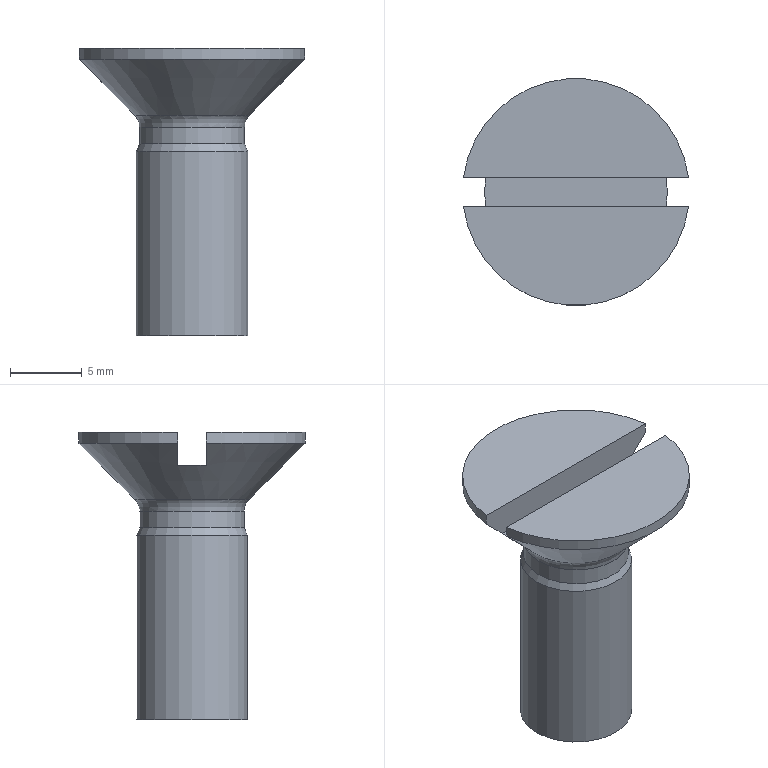Part | NX | features DATUM_CSYS 2, SKETCH 2, EXTRUDE 1, LINE 1, META 1, SWP104 1, SYMBOLIC_THREAD 1, THREADS 1 | 1 solid | 13 faces | box 15.673 x 15.8 x 20 mm | volume 1245 mm3 | plane 6 | cylinder 4 | cone 2 | torus 1 | commonest cylinder face diameters 15.8 x2 7.309 x1 7.76 x1
STEP:
#1=CARTESIAN_POINT('',(7.836,1.,0.));
#2=VERTEX_POINT('',#1);
#3=CARTESIAN_POINT('',(-7.836,1.,0.));
#4=VERTEX_POINT('',#3);
#5=CARTESIAN_POINT('',(17.3,1.,0.));
#6=DIRECTION('',(-1.,0.,0.));
#7=VECTOR('',#6,1000.);
#8=LINE('',#5,#7);
#9=EDGE_CURVE('',#2,#4,#8,.T.);
#10=ORIENTED_EDGE('',*,*,#9,.F.);
#11=CARTESIAN_POINT('',(0.,0.,0.));
#12=DIRECTION('',(0.,0.,-1.));
#13=DIRECTION('',(-1.,0.,0.));
#14=AXIS2_PLACEMENT_3D('',#11,#12,#13);
#15=CIRCLE('',#14,7.9);
#16=EDGE_CURVE('',#4,#2,#15,.T.);
#17=ORIENTED_EDGE('',*,*,#16,.F.);
#18=EDGE_LOOP('',(#10,#17));
#19=FACE_BOUND('',#18,.T.);
#20=CARTESIAN_POINT('',(0.,0.,0.));
#21=DIRECTION('',(0.,0.,-1.));
#22=DIRECTION('',(-1.,0.,0.));
#23=AXIS2_PLACEMENT_3D('',#20,#21,#22);
#24=PLANE('',#23);
#25=ADVANCED_FACE('',(#19),#24,.F.);
#26=ORIENTED_EDGE('',*,*,#16,.T.);
#27=CARTESIAN_POINT('',(7.836,1.,-0.75));
#28=VERTEX_POINT('',#27);
#29=CARTESIAN_POINT('',(7.836,1.,0.));
#30=DIRECTION('',(0.,0.,-1.));
#31=VECTOR('',#30,1000.);
#32=LINE('',#29,#31);
#33=EDGE_CURVE('',#2,#28,#32,.T.);
#34=ORIENTED_EDGE('',*,*,#33,.T.);
#35=CARTESIAN_POINT('',(-7.836,1.,-0.75));
#36=VERTEX_POINT('',#35);
#37=CARTESIAN_POINT('',(0.,0.,-0.75));
#38=DIRECTION('',(0.,0.,-1.));
#39=DIRECTION('',(-1.,0.,0.));
#40=AXIS2_PLACEMENT_3D('',#37,#38,#39);
#41=CIRCLE('',#40,7.9);
#42=EDGE_CURVE('',#36,#28,#41,.T.);
#43=ORIENTED_EDGE('',*,*,#42,.F.);
#44=CARTESIAN_POINT('',(-7.836,1.,0.));
#45=DIRECTION('',(0.,0.,-1.));
#46=VECTOR('',#45,1000.);
#47=LINE('',#44,#46);
#48=EDGE_CURVE('',#36,#4,#47,.F.);
#49=ORIENTED_EDGE('',*,*,#48,.T.);
#50=EDGE_LOOP('',(#26,#34,#43,#49));
#51=FACE_BOUND('',#50,.T.);
#52=CARTESIAN_POINT('',(0.,0.,0.));
#53=DIRECTION('',(0.,0.,-1.));
#54=DIRECTION('',(-1.,0.,0.));
#55=AXIS2_PLACEMENT_3D('',#52,#53,#54);
#56=CYLINDRICAL_SURFACE('',#55,7.9);
#57=ADVANCED_FACE('',(#51),#56,.T.);
#58=CARTESIAN_POINT('',(-3.88,0.,-7.15));
#59=VERTEX_POINT('',#58);
#60=CARTESIAN_POINT('',(0.,0.,-7.15));
#61=DIRECTION('',(0.,0.,-1.));
#62=DIRECTION('',(-1.,0.,0.));
#63=AXIS2_PLACEMENT_3D('',#60,#61,#62);
#64=CIRCLE('',#63,3.88);
#65=EDGE_CURVE('',#59,#59,#64,.T.);
#66=ORIENTED_EDGE('',*,*,#65,.F.);
#67=EDGE_LOOP('',(#66));
#68=FACE_BOUND('',#67,.T.);
#69=CARTESIAN_POINT('',(-3.655,0.,-6.65));
#70=VERTEX_POINT('',#69);
#71=CARTESIAN_POINT('',(0.,0.,-6.65));
#72=DIRECTION('',(0.,0.,-1.));
#73=DIRECTION('',(-1.,0.,0.));
#74=AXIS2_PLACEMENT_3D('',#71,#72,#73);
#75=CIRCLE('',#74,3.655);
#76=EDGE_CURVE('',#70,#70,#75,.T.);
#77=ORIENTED_EDGE('',*,*,#76,.T.);
#78=EDGE_LOOP('',(#77));
#79=FACE_BOUND('',#78,.T.);
#80=CARTESIAN_POINT('',(0.,0.,-6.65));
#81=DIRECTION('',(0.,0.,-1.));
#82=DIRECTION('',(-1.,0.,0.));
#83=AXIS2_PLACEMENT_3D('',#80,#81,#82);
#84=CONICAL_SURFACE('',#83,3.655,0.4233);
#85=ADVANCED_FACE('',(#68,#79),#84,.T.);
#86=CARTESIAN_POINT('',(-3.88,0.,-20.));
#87=VERTEX_POINT('',#86);
#88=CARTESIAN_POINT('',(0.,0.,-20.));
#89=DIRECTION('',(0.,0.,-1.));
#90=DIRECTION('',(-1.,0.,0.));
#91=AXIS2_PLACEMENT_3D('',#88,#89,#90);
#92=CIRCLE('',#91,3.88);
#93=EDGE_CURVE('',#87,#87,#92,.T.);
#94=ORIENTED_EDGE('',*,*,#93,.F.);
#95=EDGE_LOOP('',(#94));
#96=FACE_BOUND('',#95,.T.);
#97=ORIENTED_EDGE('',*,*,#65,.T.);
#98=EDGE_LOOP('',(#97));
#99=FACE_BOUND('',#98,.T.);
#100=CARTESIAN_POINT('',(0.,0.,0.));
#101=DIRECTION('',(0.,0.,-1.));
#102=DIRECTION('',(-1.,0.,0.));
#103=AXIS2_PLACEMENT_3D('',#100,#101,#102);
#104=CYLINDRICAL_SURFACE('',#103,3.88);
#105=ADVANCED_FACE('',(#96,#99),#104,.T.);
#106=ORIENTED_EDGE('',*,*,#93,.T.);
#107=EDGE_LOOP('',(#106));
#108=FACE_BOUND('',#107,.T.);
#109=CARTESIAN_POINT('',(0.,3.88,-20.));
#110=DIRECTION('',(0.,0.,1.));
#111=DIRECTION('',(1.,0.,0.));
#112=AXIS2_PLACEMENT_3D('',#109,#110,#111);
#113=PLANE('',#112);
#114=ADVANCED_FACE('',(#108),#113,.F.);
#115=CARTESIAN_POINT('',(7.836,-1.,0.));
#116=VERTEX_POINT('',#115);
#117=CARTESIAN_POINT('',(-7.836,-1.,0.));
#118=VERTEX_POINT('',#117);
#119=CARTESIAN_POINT('',(0.,0.,0.));
#120=DIRECTION('',(0.,0.,-1.));
#121=DIRECTION('',(-1.,0.,0.));
#122=AXIS2_PLACEMENT_3D('',#119,#120,#121);
#123=CIRCLE('',#122,7.9);
#124=EDGE_CURVE('',#116,#118,#123,.T.);
#125=ORIENTED_EDGE('',*,*,#124,.F.);
#126=CARTESIAN_POINT('',(17.3,-1.,0.));
#127=DIRECTION('',(-1.,0.,0.));
#128=VECTOR('',#127,1000.);
#129=LINE('',#126,#128);
#130=EDGE_CURVE('',#116,#118,#129,.T.);
#131=ORIENTED_EDGE('',*,*,#130,.T.);
#132=EDGE_LOOP('',(#125,#131));
#133=FACE_BOUND('',#132,.T.);
#134=CARTESIAN_POINT('',(0.,0.,0.));
#135=DIRECTION('',(0.,0.,-1.));
#136=DIRECTION('',(-1.,0.,0.));
#137=AXIS2_PLACEMENT_3D('',#134,#135,#136);
#138=PLANE('',#137);
#139=ADVANCED_FACE('',(#133),#138,.F.);
#140=ORIENTED_EDGE('',*,*,#124,.T.);
#141=CARTESIAN_POINT('',(-7.836,-1.,-0.75));
#142=VERTEX_POINT('',#141);
#143=CARTESIAN_POINT('',(-7.836,-1.,0.));
#144=DIRECTION('',(0.,0.,-1.));
#145=VECTOR('',#144,1000.);
#146=LINE('',#143,#145);
#147=EDGE_CURVE('',#118,#142,#146,.T.);
#148=ORIENTED_EDGE('',*,*,#147,.T.);
#149=CARTESIAN_POINT('',(7.836,-1.,-0.75));
#150=VERTEX_POINT('',#149);
#151=CARTESIAN_POINT('',(0.,0.,-0.75));
#152=DIRECTION('',(0.,0.,-1.));
#153=DIRECTION('',(-1.,0.,0.));
#154=AXIS2_PLACEMENT_3D('',#151,#152,#153);
#155=CIRCLE('',#154,7.9);
#156=EDGE_CURVE('',#150,#142,#155,.T.);
#157=ORIENTED_EDGE('',*,*,#156,.F.);
#158=CARTESIAN_POINT('',(7.836,-1.,0.));
#159=DIRECTION('',(0.,0.,-1.));
#160=VECTOR('',#159,1000.);
#161=LINE('',#158,#160);
#162=EDGE_CURVE('',#150,#116,#161,.F.);
#163=ORIENTED_EDGE('',*,*,#162,.T.);
#164=EDGE_LOOP('',(#140,#148,#157,#163));
#165=FACE_BOUND('',#164,.T.);
#166=CARTESIAN_POINT('',(0.,0.,0.));
#167=DIRECTION('',(0.,0.,-1.));
#168=DIRECTION('',(-1.,0.,0.));
#169=AXIS2_PLACEMENT_3D('',#166,#167,#168);
#170=CYLINDRICAL_SURFACE('',#169,7.9);
#171=ADVANCED_FACE('',(#165),#170,.T.);
#172=CARTESIAN_POINT('',(-4.,0.,-4.65));
#173=VERTEX_POINT('',#172);
#174=CARTESIAN_POINT('',(0.,0.,-4.65));
#175=DIRECTION('',(0.,0.,-1.));
#176=DIRECTION('',(-1.,0.,0.));
#177=AXIS2_PLACEMENT_3D('',#174,#175,#176);
#178=CIRCLE('',#177,4.);
#179=EDGE_CURVE('',#173,#173,#178,.T.);
#180=ORIENTED_EDGE('',*,*,#179,.F.);
#181=EDGE_LOOP('',(#180));
#182=FACE_BOUND('',#181,.T.);
#183=CARTESIAN_POINT('',(-6.271,-1.,-2.3));
#184=VERTEX_POINT('',#183);
#185=CARTESIAN_POINT('',(-6.271,1.,-2.3));
#186=VERTEX_POINT('',#185);
#187=CARTESIAN_POINT('',(0.,0.,-2.3));
#188=DIRECTION('',(0.,0.,-1.));
#189=DIRECTION('',(0.,1.,0.));
#190=AXIS2_PLACEMENT_3D('',#187,#188,#189);
#191=CIRCLE('',#190,6.35);
#192=EDGE_CURVE('',#184,#186,#191,.T.);
#193=ORIENTED_EDGE('',*,*,#192,.T.);
#194=CARTESIAN_POINT('',(-6.271,1.,-2.3));
#195=CARTESIAN_POINT('',(-6.793,1.,-1.784));
#196=CARTESIAN_POINT('',(-7.315,1.,-1.267));
#197=CARTESIAN_POINT('',(-7.836,1.,-0.75));
#198=B_SPLINE_CURVE_WITH_KNOTS('',3,(#194,#195,#196,#197),.UNSPECIFIED.,.F.,.F.,(4,4),(0.03236,0.03456),.UNSPECIFIED.);
#199=EDGE_CURVE('',#186,#36,#198,.T.);
#200=ORIENTED_EDGE('',*,*,#199,.T.);
#201=ORIENTED_EDGE('',*,*,#42,.T.);
#202=CARTESIAN_POINT('',(6.271,1.,-2.3));
#203=VERTEX_POINT('',#202);
#204=CARTESIAN_POINT('',(7.836,1.,-0.75));
#205=CARTESIAN_POINT('',(7.315,1.,-1.267));
#206=CARTESIAN_POINT('',(6.793,1.,-1.784));
#207=CARTESIAN_POINT('',(6.271,1.,-2.3));
#208=B_SPLINE_CURVE_WITH_KNOTS('',3,(#204,#205,#206,#207),.UNSPECIFIED.,.F.,.F.,(4,4),(0.0135,0.0157),.UNSPECIFIED.);
#209=EDGE_CURVE('',#28,#203,#208,.T.);
#210=ORIENTED_EDGE('',*,*,#209,.T.);
#211=CARTESIAN_POINT('',(6.271,-1.,-2.3));
#212=VERTEX_POINT('',#211);
#213=CARTESIAN_POINT('',(0.,0.,-2.3));
#214=DIRECTION('',(0.,0.,-1.));
#215=DIRECTION('',(0.,1.,0.));
#216=AXIS2_PLACEMENT_3D('',#213,#214,#215);
#217=CIRCLE('',#216,6.35);
#218=EDGE_CURVE('',#203,#212,#217,.T.);
#219=ORIENTED_EDGE('',*,*,#218,.T.);
#220=CARTESIAN_POINT('',(6.271,-1.,-2.3));
#221=CARTESIAN_POINT('',(6.793,-1.,-1.784));
#222=CARTESIAN_POINT('',(7.315,-1.,-1.267));
#223=CARTESIAN_POINT('',(7.836,-1.,-0.75));
#224=B_SPLINE_CURVE_WITH_KNOTS('',3,(#220,#221,#222,#223),.UNSPECIFIED.,.F.,.F.,(4,4),(0.03236,0.03456),.UNSPECIFIED.);
#225=EDGE_CURVE('',#212,#150,#224,.T.);
#226=ORIENTED_EDGE('',*,*,#225,.T.);
#227=ORIENTED_EDGE('',*,*,#156,.T.);
#228=CARTESIAN_POINT('',(-7.836,-1.,-0.75));
#229=CARTESIAN_POINT('',(-7.315,-1.,-1.267));
#230=CARTESIAN_POINT('',(-6.793,-1.,-1.784));
#231=CARTESIAN_POINT('',(-6.271,-1.,-2.3));
#232=B_SPLINE_CURVE_WITH_KNOTS('',3,(#228,#229,#230,#231),.UNSPECIFIED.,.F.,.F.,(4,4),(0.0135,0.0157),.UNSPECIFIED.);
#233=EDGE_CURVE('',#142,#184,#232,.T.);
#234=ORIENTED_EDGE('',*,*,#233,.T.);
#235=EDGE_LOOP('',(#193,#200,#201,#210,#219,#226,#227,#234));
#236=FACE_BOUND('',#235,.T.);
#237=CARTESIAN_POINT('',(0.,0.,-0.75));
#238=DIRECTION('',(0.,0.,1.));
#239=DIRECTION('',(1.,0.,0.));
#240=AXIS2_PLACEMENT_3D('',#237,#238,#239);
#241=CONICAL_SURFACE('',#240,7.9,0.7854);
#242=ADVANCED_FACE('',(#182,#236),#241,.T.);
#243=CARTESIAN_POINT('',(-3.655,0.,-5.484));
#244=VERTEX_POINT('',#243);
#245=CARTESIAN_POINT('',(0.,0.,-5.484));
#246=DIRECTION('',(0.,0.,-1.));
#247=DIRECTION('',(-1.,0.,0.));
#248=AXIS2_PLACEMENT_3D('',#245,#246,#247);
#249=CIRCLE('',#248,3.655);
#250=EDGE_CURVE('',#244,#244,#249,.T.);
#251=ORIENTED_EDGE('',*,*,#250,.F.);
#252=EDGE_LOOP('',(#251));
#253=FACE_BOUND('',#252,.T.);
#254=ORIENTED_EDGE('',*,*,#179,.T.);
#255=EDGE_LOOP('',(#254));
#256=FACE_BOUND('',#255,.T.);
#257=CARTESIAN_POINT('',(0.,0.,-5.484));
#258=DIRECTION('',(0.,0.,-1.));
#259=DIRECTION('',(-1.,0.,0.));
#260=AXIS2_PLACEMENT_3D('',#257,#258,#259);
#261=TOROIDAL_SURFACE('',#260,4.834,1.179);
#262=ADVANCED_FACE('',(#253,#256),#261,.F.);
#263=ORIENTED_EDGE('',*,*,#76,.F.);
#264=EDGE_LOOP('',(#263));
#265=FACE_BOUND('',#264,.T.);
#266=ORIENTED_EDGE('',*,*,#250,.T.);
#267=EDGE_LOOP('',(#266));
#268=FACE_BOUND('',#267,.T.);
#269=CARTESIAN_POINT('',(0.,0.,0.));
#270=DIRECTION('',(0.,0.,-1.));
#271=DIRECTION('',(-1.,0.,0.));
#272=AXIS2_PLACEMENT_3D('',#269,#270,#271);
#273=CYLINDRICAL_SURFACE('',#272,3.655);
#274=ADVANCED_FACE('',(#265,#268),#273,.T.);
#275=ORIENTED_EDGE('',*,*,#9,.T.);
#276=ORIENTED_EDGE('',*,*,#48,.F.);
#277=ORIENTED_EDGE('',*,*,#199,.F.);
#278=CARTESIAN_POINT('',(17.3,1.,-2.3));
#279=DIRECTION('',(-1.,0.,0.));
#280=VECTOR('',#279,1000.);
#281=LINE('',#278,#280);
#282=EDGE_CURVE('',#203,#186,#281,.T.);
#283=ORIENTED_EDGE('',*,*,#282,.F.);
#284=ORIENTED_EDGE('',*,*,#209,.F.);
#285=ORIENTED_EDGE('',*,*,#33,.F.);
#286=EDGE_LOOP('',(#275,#276,#277,#283,#284,#285));
#287=FACE_BOUND('',#286,.T.);
#288=CARTESIAN_POINT('',(17.3,1.,0.));
#289=DIRECTION('',(0.,1.,0.));
#290=DIRECTION('',(0.,0.,1.));
#291=AXIS2_PLACEMENT_3D('',#288,#289,#290);
#292=PLANE('',#291);
#293=ADVANCED_FACE('',(#287),#292,.F.);
#294=ORIENTED_EDGE('',*,*,#282,.T.);
#295=ORIENTED_EDGE('',*,*,#192,.F.);
#296=CARTESIAN_POINT('',(17.3,-1.,-2.3));
#297=DIRECTION('',(-1.,0.,0.));
#298=VECTOR('',#297,1000.);
#299=LINE('',#296,#298);
#300=EDGE_CURVE('',#212,#184,#299,.T.);
#301=ORIENTED_EDGE('',*,*,#300,.F.);
#302=ORIENTED_EDGE('',*,*,#218,.F.);
#303=EDGE_LOOP('',(#294,#295,#301,#302));
#304=FACE_BOUND('',#303,.T.);
#305=CARTESIAN_POINT('',(17.3,0.,-2.3));
#306=DIRECTION('',(0.,0.,-1.));
#307=DIRECTION('',(0.,1.,0.));
#308=AXIS2_PLACEMENT_3D('',#305,#306,#307);
#309=PLANE('',#308);
#310=ADVANCED_FACE('',(#304),#309,.F.);
#311=ORIENTED_EDGE('',*,*,#130,.F.);
#312=ORIENTED_EDGE('',*,*,#162,.F.);
#313=ORIENTED_EDGE('',*,*,#225,.F.);
#314=ORIENTED_EDGE('',*,*,#300,.T.);
#315=ORIENTED_EDGE('',*,*,#233,.F.);
#316=ORIENTED_EDGE('',*,*,#147,.F.);
#317=EDGE_LOOP('',(#311,#312,#313,#314,#315,#316));
#318=FACE_BOUND('',#317,.T.);
#319=CARTESIAN_POINT('',(17.3,-1.,-2.3));
#320=DIRECTION('',(0.,-1.,0.));
#321=DIRECTION('',(0.,0.,-1.));
#322=AXIS2_PLACEMENT_3D('',#319,#320,#321);
#323=PLANE('',#322);
#324=ADVANCED_FACE('',(#318),#323,.F.);
#325=CLOSED_SHELL('',(#25,#57,#85,#105,#114,#139,#171,#242,#262,#274,#293,#310,#324));
#326=MANIFOLD_SOLID_BREP('',#325);
#327=(LENGTH_UNIT()NAMED_UNIT(*)SI_UNIT(.MILLI.,.METRE.));
#328=UNCERTAINTY_MEASURE_WITH_UNIT(LENGTH_MEASURE(0.0508),#327,'','');
#329=(NAMED_UNIT(*)PLANE_ANGLE_UNIT()SI_UNIT($,.RADIAN.));
#330=(NAMED_UNIT(*)SI_UNIT($,.STERADIAN.)SOLID_ANGLE_UNIT());
#331=(GEOMETRIC_REPRESENTATION_CONTEXT(3)GLOBAL_UNCERTAINTY_ASSIGNED_CONTEXT((#328))GLOBAL_UNIT_ASSIGNED_CONTEXT((#327,#329,#330))REPRESENTATION_CONTEXT('',''));
#332=ADVANCED_BREP_SHAPE_REPRESENTATION('',(#326),#331);